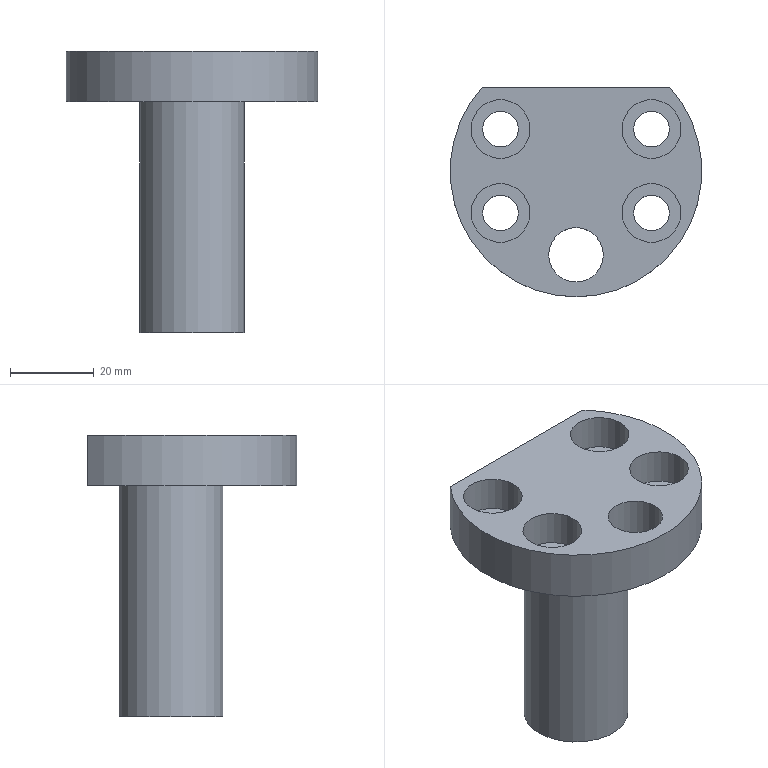NC program | NX | posted with a generic post | part box 60 x 50 x 67 mm
Whole program:
N10 G17 G21 G94 G90
(DRILLING , TOOL : ZXZ)
N12 T01 M6
N14 G54
N16 G17 G0 G90 X-18. Y10. S3000 M3
N18 G43 Z30. H1
N20 G94 G81 G98 Z-1. F200. R3.
N22 Y-10.
N24 X0. Y-20.
N26 X18. Y-10.
N28 Y10.
N30 G80
N32 G0 X18. Y10. Z30.
N34 M5
(DRILLING_COPY , TOOL : 8.5ZT)
N36 T02 M6
N38 G54
N40 G17 G0 G90 X-18. Y10. S1200 M3
N42 G43 Z30. H2
N44 G94 G83 G98 Z-16.054 F120. Q2. R3.
N46 X18.
N48 Y-10.
N50 X-18.
N52 G80
N54 G0 X-18. Y-10. Z30.
N56 M5
(DRILLING_COPY_COPY , TOOL : 13.0ZT)
N58 T03 M6
N60 G54
N62 G17 G0 G90 X0. Y-20. S600 M3
N64 G43 Z30. H3
N66 G94 G83 G98 Z-17.406 F120. Q2. R3.
N68 G80
N70 G0 X0. Y-20. Z30.
N72 M5
(HOLE_MILLING , TOOL : D10)
N74 T10 M6
N76 G54
N78 G17 G0 G90 X-18. Y10. S3000 M3
N80 G43 Z30. H10
N82 Z0.5
N84 G94 G3 X-17. Y9. R1. F2000.
N86 X-16. Y10. R1.
N88 X-16. Y10. Z0.28 I-2. J0.
N90 X-16. Y10. Z0.06 I-2. J0.
N92 X-16. Y10. Z-0.16 I-2. J0.
N94 X-16. Y10. Z-0.38 I-2. J0.
N96 X-16. Y10. Z-0.6 I-2. J0.
N98 X-16. Y10. Z-0.82 I-2. J0.
N100 X-16. Y10. Z-1.04 I-2. J0.
N102 X-16. Y10. Z-1.26 I-2. J0.
N104 X-16. Y10. Z-1.48 I-2. J0.
N106 X-16. Y10. Z-1.7 I-2. J0.
N108 X-16. Y10. Z-1.92 I-2. J0.
N110 X-16. Y10. Z-2.14 I-2. J0.
N112 X-16. Y10. Z-2.36 I-2. J0.
N114 X-16. Y10. Z-2.58 I-2. J0.
N116 X-16. Y10. Z-2.8 I-2. J0.
N118 X-16. Y10. Z-3.02 I-2. J0.
N120 X-16. Y10. Z-3.24 I-2. J0.
N122 X-16. Y10. Z-3.46 I-2. J0.
N124 X-16. Y10. Z-3.68 I-2. J0.
N126 X-16. Y10. Z-3.9 I-2. J0.
N128 X-16. Y10. Z-4.12 I-2. J0.
N130 X-16. Y10. Z-4.34 I-2. J0.
N132 X-16. Y10. Z-4.56 I-2. J0.
N134 X-16. Y10. Z-4.78 I-2. J0.
N136 X-16. Y10. Z-5. I-2. J0.
N138 X-16. Y10. Z-5.22 I-2. J0.
N140 X-16. Y10. Z-5.44 I-2. J0.
N142 X-16. Y10. Z-5.66 I-2. J0.
N144 X-16. Y10. Z-5.88 I-2. J0.
N146 X-16. Y10. Z-6.1 I-2. J0.
N148 X-16. Y10. Z-6.32 I-2. J0.
N150 X-16. Y10. Z-6.54 I-2. J0.
N152 X-16. Y10. Z-6.76 I-2. J0.
N154 X-16. Y10. Z-6.98 I-2. J0.
N156 X-16. Y10. Z-7.2 I-2. J0.
N158 X-16. Y10. Z-7.42 I-2. J0.
N160 X-16. Y10. Z-7.64 I-2. J0.
N162 X-16. Y10. Z-7.86 I-2. J0.
N164 X-16. Y10. Z-8.08 I-2. J0.
N166 X-16. Y10. Z-8.3 I-2. J0.
N168 X-16.317 Y8.919 Z-8.5 R-2.
N170 X-16.919 Y11.683 R2.
N172 X-16.317 Y8.919 R-2.
N174 X-16.618 Y10.301 R1.
N176 X-18. Y10. R1.
N178 G0 Z30.
N180 Y-10.
N182 Z0.5
N184 G3 X-17. Y-11. R1.
N186 X-16. Y-10. R1.
N188 X-16. Y-10. Z0.28 I-2. J0.
N190 X-16. Y-10. Z0.06 I-2. J0.
N192 X-16. Y-10. Z-0.16 I-2. J0.
N194 X-16. Y-10. Z-0.38 I-2. J0.
N196 X-16. Y-10. Z-0.6 I-2. J0.
N198 X-16. Y-10. Z-0.82 I-2. J0.
N200 X-16. Y-10. Z-1.04 I-2. J0.
N202 X-16. Y-10. Z-1.26 I-2. J0.
N204 X-16. Y-10. Z-1.48 I-2. J0.
N206 X-16. Y-10. Z-1.7 I-2. J0.
N208 X-16. Y-10. Z-1.92 I-2. J0.
N210 X-16. Y-10. Z-2.14 I-2. J0.
N212 X-16. Y-10. Z-2.36 I-2. J0.
N214 X-16. Y-10. Z-2.58 I-2. J0.
N216 X-16. Y-10. Z-2.8 I-2. J0.
N218 X-16. Y-10. Z-3.02 I-2. J0.
N220 X-16. Y-10. Z-3.24 I-2. J0.
N222 X-16. Y-10. Z-3.46 I-2. J0.
N224 X-16. Y-10. Z-3.68 I-2. J0.
N226 X-16. Y-10. Z-3.9 I-2. J0.
N228 X-16. Y-10. Z-4.12 I-2. J0.
N230 X-16. Y-10. Z-4.34 I-2. J0.
N232 X-16. Y-10. Z-4.56 I-2. J0.
N234 X-16. Y-10. Z-4.78 I-2. J0.
N236 X-16. Y-10. Z-5. I-2. J0.
N238 X-16. Y-10. Z-5.22 I-2. J0.
N240 X-16. Y-10. Z-5.44 I-2. J0.
N242 X-16. Y-10. Z-5.66 I-2. J0.
N244 X-16. Y-10. Z-5.88 I-2. J0.
N246 X-16. Y-10. Z-6.1 I-2. J0.
N248 X-16. Y-10. Z-6.32 I-2. J0.
N250 X-16. Y-10. Z-6.54 I-2. J0.
N252 X-16. Y-10. Z-6.76 I-2. J0.
N254 X-16. Y-10. Z-6.98 I-2. J0.
N256 X-16. Y-10. Z-7.2 I-2. J0.
N258 X-16. Y-10. Z-7.42 I-2. J0.
N260 X-16. Y-10. Z-7.64 I-2. J0.
N262 X-16. Y-10. Z-7.86 I-2. J0.
N264 X-16. Y-10. Z-8.08 I-2. J0.
N266 X-16. Y-10. Z-8.3 I-2. J0.
N268 X-16.317 Y-11.081 Z-8.5 R-2.
N270 X-16.919 Y-8.317 R2.
N272 X-16.317 Y-11.081 R-2.
N274 X-16.618 Y-9.699 R1.
N276 X-18. Y-10. R1.
N278 G0 Z30.
N280 X18.
N282 Z0.5
N284 G3 X19. Y-11. R1.
N286 X20. Y-10. R1.
N288 X20. Y-10. Z0.28 I-2. J0.
N290 X20. Y-10. Z0.06 I-2. J0.
N292 X20. Y-10. Z-0.16 I-2. J0.
N294 X20. Y-10. Z-0.38 I-2. J0.
N296 X20. Y-10. Z-0.6 I-2. J0.
N298 X20. Y-10. Z-0.82 I-2. J0.
N300 X20. Y-10. Z-1.04 I-2. J0.
N302 X20. Y-10. Z-1.26 I-2. J0.
N304 X20. Y-10. Z-1.48 I-2. J0.
N306 X20. Y-10. Z-1.7 I-2. J0.
N308 X20. Y-10. Z-1.92 I-2. J0.
N310 X20. Y-10. Z-2.14 I-2. J0.
N312 X20. Y-10. Z-2.36 I-2. J0.
N314 X20. Y-10. Z-2.58 I-2. J0.
N316 X20. Y-10. Z-2.8 I-2. J0.
N318 X20. Y-10. Z-3.02 I-2. J0.
N320 X20. Y-10. Z-3.24 I-2. J0.
N322 X20. Y-10. Z-3.46 I-2. J0.
N324 X20. Y-10. Z-3.68 I-2. J0.
N326 X20. Y-10. Z-3.9 I-2. J0.
N328 X20. Y-10. Z-4.12 I-2. J0.
N330 X20. Y-10. Z-4.34 I-2. J0.
N332 X20. Y-10. Z-4.56 I-2. J0.
N334 X20. Y-10. Z-4.78 I-2. J0.
N336 X20. Y-10. Z-5. I-2. J0.
N338 X20. Y-10. Z-5.22 I-2. J0.
N340 X20. Y-10. Z-5.44 I-2. J0.
N342 X20. Y-10. Z-5.66 I-2. J0.
N344 X20. Y-10. Z-5.88 I-2. J0.
N346 X20. Y-10. Z-6.1 I-2. J0.
N348 X20. Y-10. Z-6.32 I-2. J0.
N350 X20. Y-10. Z-6.54 I-2. J0.
N352 X20. Y-10. Z-6.76 I-2. J0.
N354 X20. Y-10. Z-6.98 I-2. J0.
N356 X20. Y-10. Z-7.2 I-2. J0.
N358 X20. Y-10. Z-7.42 I-2. J0.
N360 X20. Y-10. Z-7.64 I-2. J0.
N362 X20. Y-10. Z-7.86 I-2. J0.
N364 X20. Y-10. Z-8.08 I-2. J0.
N366 X20. Y-10. Z-8.3 I-2. J0.
N368 X19.683 Y-11.081 Z-8.5 R-2.
N370 X19.081 Y-8.317 R2.
N372 X19.683 Y-11.081 R-2.
N374 X19.382 Y-9.699 R1.
N376 X18. Y-10. R1.
N378 G0 Z30.
N380 Y10.
N382 Z0.5
N384 G3 X19. Y9. R1.
N386 X20. Y10. R1.
N388 X20. Y10. Z0.28 I-2. J0.
N390 X20. Y10. Z0.06 I-2. J0.
N392 X20. Y10. Z-0.16 I-2. J0.
N394 X20. Y10. Z-0.38 I-2. J0.
N396 X20. Y10. Z-0.6 I-2. J0.
N398 X20. Y10. Z-0.82 I-2. J0.
N400 X20. Y10. Z-1.04 I-2. J0.
N402 X20. Y10. Z-1.26 I-2. J0.
N404 X20. Y10. Z-1.48 I-2. J0.
N406 X20. Y10. Z-1.7 I-2. J0.
N408 X20. Y10. Z-1.92 I-2. J0.
N410 X20. Y10. Z-2.14 I-2. J0.
N412 X20. Y10. Z-2.36 I-2. J0.
N414 X20. Y10. Z-2.58 I-2. J0.
N416 X20. Y10. Z-2.8 I-2. J0.
N418 X20. Y10. Z-3.02 I-2. J0.
N420 X20. Y10. Z-3.24 I-2. J0.
N422 X20. Y10. Z-3.46 I-2. J0.
N424 X20. Y10. Z-3.68 I-2. J0.
N426 X20. Y10. Z-3.9 I-2. J0.
N428 X20. Y10. Z-4.12 I-2. J0.
N430 X20. Y10. Z-4.34 I-2. J0.
N432 X20. Y10. Z-4.56 I-2. J0.
N434 X20. Y10. Z-4.78 I-2. J0.
N436 X20. Y10. Z-5. I-2. J0.
N438 X20. Y10. Z-5.22 I-2. J0.
N440 X20. Y10. Z-5.44 I-2. J0.
N442 X20. Y10. Z-5.66 I-2. J0.
N444 X20. Y10. Z-5.88 I-2. J0.
N446 X20. Y10. Z-6.1 I-2. J0.
N448 X20. Y10. Z-6.32 I-2. J0.
N450 X20. Y10. Z-6.54 I-2. J0.
N452 X20. Y10. Z-6.76 I-2. J0.
N454 X20. Y10. Z-6.98 I-2. J0.
N456 X20. Y10. Z-7.2 I-2. J0.
N458 X20. Y10. Z-7.42 I-2. J0.
N460 X20. Y10. Z-7.64 I-2. J0.
N462 X20. Y10. Z-7.86 I-2. J0.
N464 X20. Y10. Z-8.08 I-2. J0.
N466 X20. Y10. Z-8.3 I-2. J0.
N468 X19.683 Y8.919 Z-8.5 R-2.
N470 X19.081 Y11.683 R2.
N472 X19.683 Y8.919 R-2.
N474 X19.382 Y10.301 R1.
N476 X18. Y10. R1.
N478 G0 Z30.
N480 M5
(ZLEVEL_PROFILE_1_COPY_1 , TOOL : D6A45)
N482 T07 M6
N484 G54
N486 G17 G0 G90 X-22.797 Y-8.887 S7500 M3
N488 G43 Z30. H7
N490 Z0.
N492 G94 G1 Z-1. F1000.
N494 X-23.824 Y-9.48
N496 G3 X-24.124 Y-10. R0.6
N498 X-18. Y-16.124 R6.124
N500 X-24.124 Y-10. R-6.124
N502 X-23.824 Y-10.52 R0.6
N504 G1 X-22.797 Y-11.113
N506 Z0.
N508 G0 Z30.
N510 X22.797
N512 Z0.
N514 G1 Z-1.
N516 X23.824 Y-10.52
N518 G3 X24.124 Y-10. R0.6
N520 X18. Y-3.876 R6.124
N522 X24.124 Y-10. R-6.124
N524 X23.824 Y-9.48 R0.6
N526 G1 X22.797 Y-8.887
N528 Z0.
N530 G0 Z30.
N532 X-16.887 Y14.797
N534 Z0.
N536 G1 Z-1.
N538 X-17.48 Y15.824
N540 G3 X-18. Y16.124 R0.6
N542 X-24.124 Y10. R6.124
N544 X-18. Y16.124 R-6.124
N546 X-18.52 Y15.824 R0.6
N548 G1 X-19.113 Y14.797
N550 Z0.
N552 G0 Z30.
N554 X19.113
N556 Z0.
N558 G1 Z-1.
N560 X18.52 Y15.824
N562 G3 X18. Y16.124 R0.6
N564 X11.876 Y10. R6.124
N566 X18. Y16.124 R-6.124
N568 X17.48 Y15.824 R0.6
N570 G1 X16.887 Y14.797
N572 Z0.
N574 G0 Z30.
N576 X-1.123 Y-24.279
N578 Z0.
N580 G1 Z-1.
N582 X-0.52 Y-25.324
N584 G3 X0. Y-25.624 R0.6
N586 X5.624 Y-20. R5.624
N588 X0. Y-25.624 R-5.624
N590 X0.52 Y-25.324 R0.6
N592 G1 X1.123 Y-24.279
N594 Z0.
N596 G0 Z30.
N598 M5
N600 M2